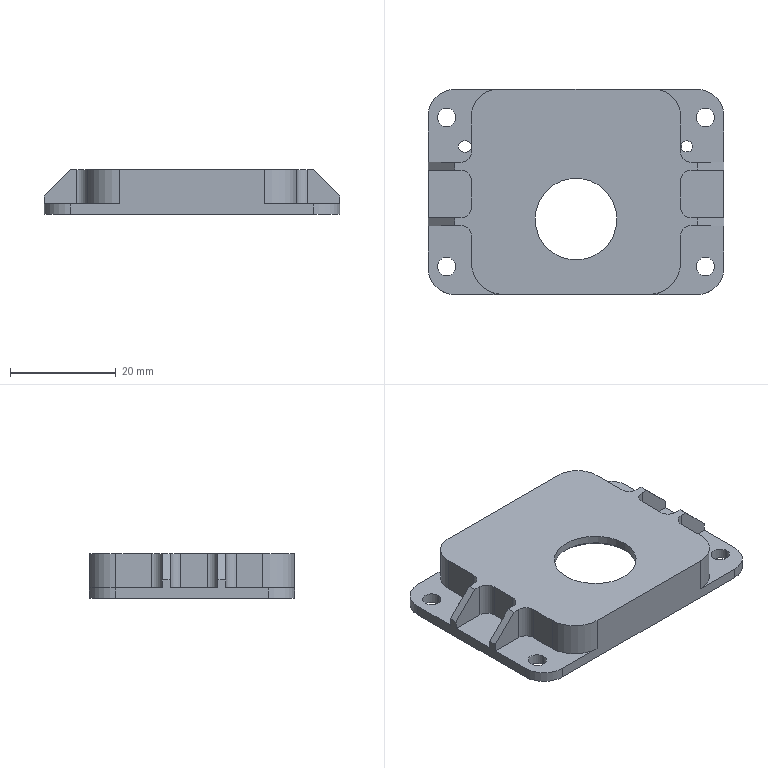NC program | NX | posted with a generic post | part box 56 x 38.85 x 8.5 mm
Lines 2523 to 3190 of 3190:
(ZLEVEL_PROFILE_COPY , TOOL : D1.5)
N5008 T20 M6
N5010 G54
N5012 G17 G0 G90 X21.294 Y8.344 S9500 M3
N5014 G43 Z30. H20
N5016 Z0.5
N5018 G94 G1 X21.435 Y8.379 Z0.492 F1000.
N5020 X21.546 Y8.537 Z0.482
N5022 Y8.646 Z0.477
N5024 X21.514 Y8.79 Z0.469
N5026 X21.432 Y8.874 Z0.463
N5028 X21.29 Y8.909 Z0.455
N5030 X21.229 Y8.925 Z0.452
N5032 X20.776 Z0.428
N5034 X20.748 Y8.916 Z0.426
N5036 X20.613 Y8.917 Z0.419
N5038 X20.521 Y8.854 Z0.413
N5040 X20.426 Y8.6 Z0.399
N5042 X20.494 Y8.427 Z0.39
N5044 X20.615 Y8.365 Z0.382
N5046 X20.775 Y8.325 Z0.374
N5048 X21.218 Z0.351
N5050 X21.435 Y8.379 Z0.339
N5052 X21.546 Y8.537 Z0.329
N5054 Y8.646 Z0.323
N5056 X21.514 Y8.79 Z0.315
N5058 X21.432 Y8.874 Z0.309
N5060 X21.29 Y8.909 Z0.301
N5062 X21.229 Y8.925 Z0.298
N5064 X20.776 Z0.274
N5066 X20.748 Y8.916 Z0.273
N5068 X20.613 Y8.917 Z0.266
N5070 X20.521 Y8.854 Z0.26
N5072 X20.426 Y8.6 Z0.246
N5074 X20.494 Y8.427 Z0.236
N5076 X20.615 Y8.365 Z0.229
N5078 X20.775 Y8.325 Z0.22
N5080 X21.218 Z0.197
N5082 X21.435 Y8.379 Z0.185
N5084 X21.546 Y8.537 Z0.175
N5086 Y8.646 Z0.169
N5088 X21.514 Y8.79 Z0.162
N5090 X21.432 Y8.874 Z0.156
N5092 X21.29 Y8.909 Z0.148
N5094 X21.229 Y8.925 Z0.145
N5096 X20.776 Z0.121
N5098 X20.748 Y8.916 Z0.119
N5100 X20.613 Y8.917 Z0.112
N5102 X20.521 Y8.854 Z0.106
N5104 X20.426 Y8.6 Z0.092
N5106 X20.494 Y8.427 Z0.082
N5108 X20.615 Y8.365 Z0.075
N5110 X20.775 Y8.325 Z0.067
N5112 X21.218 Z0.043
N5114 X21.435 Y8.379 Z0.032
N5116 X21.546 Y8.537 Z0.022
N5118 Y8.646 Z0.016
N5120 X21.514 Y8.79 Z0.008
N5122 X21.432 Y8.874 Z0.002
N5124 X21.29 Y8.909 Z-0.006
N5126 X21.229 Y8.925 Z-0.009
N5128 X20.776 Z-0.033
N5130 X20.748 Y8.916 Z-0.034
N5132 X20.613 Y8.917 Z-0.041
N5134 X20.521 Y8.854 Z-0.047
N5136 X20.426 Y8.6 Z-0.061
N5138 X20.494 Y8.427 Z-0.071
N5140 X20.615 Y8.365 Z-0.078
N5142 X20.775 Y8.325 Z-0.087
N5144 X21.026 Z-0.1
N5146 X21.218
N5148 X21.435 Y8.379
N5150 X21.546 Y8.537
N5152 Y8.646
N5154 G3 X21.29 Y8.909 R0.345
N5156 G1 X21.229 Y8.925
N5158 X20.776
N5160 X20.748 Y8.916
N5162 G3 X20.615 Y8.365 R0.291
N5164 G1 X20.775 Y8.325
N5166 X21.026
N5168 X21.258 Y8.337 Z-0.111
N5170 X21.29 Y8.343 Z-0.113
N5172 X21.456 Y8.416 Z-0.121
N5174 X21.503 Y8.475 Z-0.125
N5176 X21.543 Y8.58 Z-0.13
N5178 X21.546 Y8.63 Z-0.133
N5180 X21.527 Y8.728 Z-0.138
N5182 X21.477 Y8.807 Z-0.142
N5184 X21.449 Y8.843 Z-0.144
N5186 X21.41 Y8.865 Z-0.146
N5188 X21.327 Y8.902 Z-0.15
N5190 X21.272 Y8.911 Z-0.153
N5192 X21.062 Y8.925 Z-0.163
N5194 X20.796 Z-0.175
N5196 X20.612 Y8.879 Z-0.184
N5198 X20.548 Y8.842 Z-0.188
N5200 X20.475 Y8.732 Z-0.194
N5202 X20.457 Y8.6 Z-0.2
N5204 G3 X20.615 Y8.365 R0.291
N5206 G1 X20.775 Y8.325
N5208 X21.026
N5210 X21.257 Y8.337 Z-0.211
N5212 X21.29 Y8.343 Z-0.213
N5214 X21.456 Y8.416 Z-0.221
N5216 X21.503 Y8.475 Z-0.225
N5218 X21.543 Y8.579 Z-0.23
N5220 X21.545 Y8.663 Z-0.234
N5222 X21.527 Y8.728 Z-0.238
N5224 X21.477 Y8.81 Z-0.242
N5226 X21.447 Y8.845 Z-0.244
N5228 X21.409 Y8.866 Z-0.246
N5230 X21.327 Y8.902 Z-0.25
N5232 X21.271 Y8.911 Z-0.253
N5234 X21.062 Y8.925 Z-0.263
N5236 X20.796 Z-0.275
N5238 X20.612 Y8.879 Z-0.284
N5240 X20.549 Y8.842 Z-0.288
N5242 X20.475 Y8.731 Z-0.294
N5244 X20.457 Y8.6 Z-0.3
N5246 G3 X20.615 Y8.365 R0.291
N5248 G1 X20.775 Y8.325
N5250 X21.026
N5252 X21.257 Y8.337 Z-0.311
N5254 X21.29 Y8.343 Z-0.313
N5256 X21.455 Y8.416 Z-0.321
N5258 X21.502 Y8.475 Z-0.325
N5260 X21.546 Y8.63 Z-0.333
N5262 X21.527 Y8.728 Z-0.338
N5264 X21.48 Y8.804 Z-0.342
N5266 X21.453 Y8.839 Z-0.344
N5268 X21.414 Y8.864 Z-0.346
N5270 X21.327 Y8.902 Z-0.35
N5272 X21.27 Y8.911 Z-0.353
N5274 X21.062 Y8.925 Z-0.363
N5276 X20.796 Z-0.375
N5278 X20.612 Y8.879 Z-0.384
N5280 X20.549 Y8.841 Z-0.388
N5282 X20.475 Y8.731 Z-0.394
N5284 X20.457 Y8.6 Z-0.4
N5286 G3 X20.615 Y8.365 R0.291
N5288 G1 X20.775 Y8.325
N5290 X21.026
N5292 X21.257 Y8.337 Z-0.411
N5294 X21.29 Y8.343 Z-0.413
N5296 X21.455 Y8.416 Z-0.421
N5298 X21.502 Y8.476 Z-0.425
N5300 X21.546 Y8.629 Z-0.432
N5302 X21.527 Y8.728 Z-0.438
N5304 X21.48 Y8.804 Z-0.442
N5306 X21.453 Y8.839 Z-0.444
N5308 X21.414 Y8.863 Z-0.446
N5310 X21.327 Y8.902 Z-0.45
N5312 X21.271 Y8.912 Z-0.453
N5314 X21.062 Y8.925 Z-0.463
N5316 X20.796 Z-0.475
N5318 X20.615 Y8.879 Z-0.484
N5320 X20.55 Y8.84 Z-0.488
N5322 X20.474 Y8.73 Z-0.494
N5324 X20.451 Y8.6 Z-0.5
N5326 G3 X20.709 Y8.328 R0.3
N5328 G1 X20.775 Y8.325
N5330 X21.026
N5332 X21.259 Y8.337 Z-0.511
N5334 X21.292 Y8.343 Z-0.513
N5336 X21.411 Y8.388 Z-0.518
N5338 X21.464 Y8.415 Z-0.521
N5340 X21.51 Y8.475 Z-0.525
N5342 X21.55 Y8.635 Z-0.533
N5344 X21.529 Y8.735 Z-0.538
N5346 X21.485 Y8.811 Z-0.541
N5348 X21.457 Y8.843 Z-0.543
N5350 X21.411 Y8.863 Z-0.546
N5352 X21.32 Y8.903 Z-0.55
N5354 X21.258 Y8.914 Z-0.553
N5356 X21.054 Y8.925 Z-0.563
N5358 X20.836 Z-0.573
N5360 X20.785 Y8.92 Z-0.575
N5362 X20.59 Y8.864 Z-0.585
N5364 X20.539 Y8.839 Z-0.588
N5366 X20.468 Y8.726 Z-0.594
N5368 X20.452 Y8.594 Z-0.6
N5370 G3 X20.709 Y8.328 R0.3
N5372 G1 X20.775 Y8.325
N5374 X21.026
N5376 X21.294 Y8.343 Z-0.613
N5378 X21.456 Y8.418 Z-0.621
N5380 X21.511 Y8.477 Z-0.625
N5382 X21.547 Y8.625 Z-0.632
N5384 X21.528 Y8.738 Z-0.638
N5386 X21.456 Y8.835 Z-0.643
N5388 X21.33 Y8.901 Z-0.65
N5390 X21.281 Y8.908 Z-0.652
N5392 X21.064 Y8.925 Z-0.663
N5394 X20.794 Z-0.675
N5396 X20.61 Y8.875 Z-0.684
N5398 X20.544 Y8.843 Z-0.688
N5400 X20.47 Y8.732 Z-0.694
N5402 X20.451 Y8.599 Z-0.7
N5404 G3 X20.709 Y8.328 R0.3
N5406 G1 X20.775 Y8.325
N5408 X21.026
N5410 X21.294 Y8.343 Z-0.713
N5412 X21.456 Y8.418 Z-0.721
N5414 X21.511 Y8.477 Z-0.725
N5416 X21.547 Y8.625 Z-0.732
N5418 X21.528 Y8.738 Z-0.738
N5420 X21.456 Y8.835 Z-0.743
N5422 X21.33 Y8.901 Z-0.75
N5424 X21.281 Y8.908 Z-0.752
N5426 X21.064 Y8.925 Z-0.763
N5428 X20.794 Z-0.775
N5430 X20.61 Y8.875 Z-0.784
N5432 X20.544 Y8.843 Z-0.788
N5434 X20.47 Y8.732 Z-0.794
N5436 X20.451 Y8.599 Z-0.8
N5438 G3 X20.709 Y8.328 R0.3
N5440 G1 X20.776 Y8.325
N5442 X21.026
N5444 X21.26 Y8.338 Z-0.811
N5446 X21.294 Y8.343 Z-0.813
N5448 X21.411 Y8.388 Z-0.818
N5450 X21.465 Y8.415 Z-0.821
N5452 X21.511 Y8.477 Z-0.825
N5454 X21.55 Y8.636 Z-0.832
N5456 X21.528 Y8.738 Z-0.838
N5458 X21.457 Y8.842 Z-0.843
N5460 X21.415 Y8.862 Z-0.846
N5462 X21.33 Y8.901 Z-0.85
N5464 X21.275 Y8.909 Z-0.853
N5466 X21.064 Y8.925 Z-0.863
N5468 X20.794 Z-0.875
N5470 X20.61 Y8.875 Z-0.884
N5472 X20.544 Y8.843 Z-0.888
N5474 X20.47 Y8.732 Z-0.894
N5476 X20.451 Y8.599 Z-0.9
N5478 G3 X20.709 Y8.328 R0.3
N5480 G1 X20.776 Y8.325
N5482 X21.026
N5484 X21.26 Y8.338 Z-0.911
N5486 X21.294 Y8.343 Z-0.913
N5488 X21.411 Y8.388 Z-0.918
N5490 X21.465 Y8.415 Z-0.921
N5492 X21.511 Y8.477 Z-0.925
N5494 X21.55 Y8.636 Z-0.932
N5496 X21.528 Y8.738 Z-0.938
N5498 X21.457 Y8.842 Z-0.943
N5500 X21.415 Y8.862 Z-0.946
N5502 X21.33 Y8.901 Z-0.95
N5504 X21.275 Y8.909 Z-0.953
N5506 X21.064 Y8.925 Z-0.963
N5508 X20.794 Z-0.975
N5510 X20.61 Y8.875 Z-0.984
N5512 X20.544 Y8.843 Z-0.988
N5514 X20.47 Y8.732 Z-0.994
N5516 X20.451 Y8.599 Z-1.
N5518 G3 X20.709 Y8.328 R0.3
N5520 G1 X20.776 Y8.325
N5522 X21.026
N5524 X21.26 Y8.338 Z-1.011
N5526 X21.294 Y8.344 Z-1.013
N5528 X21.41 Y8.388 Z-1.018
N5530 X21.464 Y8.415 Z-1.021
N5532 X21.511 Y8.477 Z-1.025
N5534 X21.55 Y8.636 Z-1.032
N5536 X21.528 Y8.738 Z-1.038
N5538 X21.457 Y8.842 Z-1.043
N5540 X21.33 Y8.901 Z-1.05
N5542 X21.275 Y8.911 Z-1.053
N5544 X21.064 Y8.925 Z-1.063
N5546 X20.794 Z-1.075
N5548 X20.61 Y8.875 Z-1.084
N5550 X20.544 Y8.843 Z-1.088
N5552 X20.47 Y8.732 Z-1.094
N5554 X20.451 Y8.599 Z-1.1
N5556 G3 X20.709 Y8.328 R0.3
N5558 G1 X20.776 Y8.325
N5560 X21.026
N5562 X21.26 Y8.338 Z-1.111
N5564 X21.294 Y8.344 Z-1.113
N5566 X21.41 Y8.388 Z-1.118
N5568 X21.464 Y8.415 Z-1.121
N5570 X21.511 Y8.477 Z-1.125
N5572 X21.55 Y8.636 Z-1.132
N5574 X21.528 Y8.738 Z-1.138
N5576 X21.457 Y8.842 Z-1.143
N5578 X21.33 Y8.901 Z-1.15
N5580 X21.275 Y8.911 Z-1.153
N5582 X21.064 Y8.925 Z-1.163
N5584 X20.794 Z-1.175
N5586 X20.61 Y8.875 Z-1.184
N5588 X20.544 Y8.843 Z-1.188
N5590 X20.47 Y8.732 Z-1.194
N5592 X20.451 Y8.599 Z-1.2
N5594 G3 X20.709 Y8.328 R0.3
N5596 G1 X20.776 Y8.325
N5598 X21.026
N5600 X21.259 Y8.338 Z-1.211
N5602 X21.294 Y8.344 Z-1.213
N5604 X21.41 Y8.388 Z-1.218
N5606 X21.464 Y8.415 Z-1.221
N5608 X21.511 Y8.477 Z-1.225
N5610 X21.55 Y8.636 Z-1.232
N5612 X21.528 Y8.738 Z-1.238
N5614 X21.457 Y8.842 Z-1.243
N5616 X21.33 Y8.901 Z-1.25
N5618 X21.274 Y8.91 Z-1.253
N5620 X21.064 Y8.925 Z-1.263
N5622 X20.794 Z-1.275
N5624 X20.61 Y8.875 Z-1.284
N5626 X20.544 Y8.843 Z-1.288
N5628 X20.47 Y8.732 Z-1.294
N5630 X20.451 Y8.599 Z-1.3
N5632 G3 X20.709 Y8.328 R0.3
N5634 G1 X20.776 Y8.325
N5636 X21.026
N5638 X21.259 Y8.338 Z-1.311
N5640 X21.294 Y8.344 Z-1.313
N5642 X21.41 Y8.388 Z-1.318
N5644 X21.464 Y8.415 Z-1.321
N5646 X21.511 Y8.477 Z-1.325
N5648 X21.55 Y8.636 Z-1.332
N5650 X21.528 Y8.738 Z-1.338
N5652 X21.458 Y8.842 Z-1.343
N5654 X21.33 Y8.9 Z-1.35
N5656 X21.274 Y8.91 Z-1.353
N5658 X21.064 Y8.925 Z-1.363
N5660 X20.794 Z-1.375
N5662 X20.61 Y8.875 Z-1.384
N5664 X20.544 Y8.843 Z-1.388
N5666 X20.47 Y8.732 Z-1.394
N5668 X20.451 Y8.599 Z-1.4
N5670 G3 X20.709 Y8.328 R0.3
N5672 G1 X20.776 Y8.325
N5674 X21.026
N5676 X21.294 Y8.344 Z-1.413
N5678 X21.409 Y8.389 Z-1.418
N5680 X21.464 Y8.414 Z-1.421
N5682 X21.511 Y8.477 Z-1.425
N5684 X21.55 Y8.636 Z-1.432
N5686 X21.528 Y8.738 Z-1.438
N5688 X21.458 Y8.841 Z-1.443
N5690 X21.33 Y8.9 Z-1.45
N5692 X21.273 Y8.91 Z-1.453
N5694 X21.064 Y8.925 Z-1.463
N5696 X20.794 Z-1.475
N5698 X20.61 Y8.875 Z-1.484
N5700 X20.544 Y8.843 Z-1.488
N5702 X20.47 Y8.732 Z-1.494
N5704 X20.451 Y8.599 Z-1.5
N5706 G3 X20.709 Y8.328 R0.3
N5708 G1 X20.776 Y8.325
N5710 X21.026
N5712 X21.294 Y8.344 Z-1.513
N5714 X21.409 Y8.389 Z-1.518
N5716 X21.463 Y8.414 Z-1.521
N5718 X21.511 Y8.477 Z-1.525
N5720 X21.55 Y8.636 Z-1.532
N5722 X21.528 Y8.738 Z-1.538
N5724 X21.458 Y8.841 Z-1.543
N5726 X21.33 Y8.9 Z-1.55
N5728 X21.273 Y8.91 Z-1.553
N5730 X21.064 Y8.925 Z-1.563
N5732 X20.794 Z-1.575
N5734 X20.61 Y8.875 Z-1.584
N5736 X20.544 Y8.843 Z-1.588
N5738 X20.47 Y8.732 Z-1.594
N5740 X20.451 Y8.599 Z-1.6
N5742 G3 X20.709 Y8.328 R0.3
N5744 G1 X20.776 Y8.325
N5746 X21.026
N5748 X21.294 Y8.344 Z-1.613
N5750 X21.409 Y8.389 Z-1.618
N5752 X21.463 Y8.414 Z-1.621
N5754 X21.511 Y8.477 Z-1.625
N5756 X21.55 Y8.636 Z-1.632
N5758 X21.528 Y8.738 Z-1.638
N5760 X21.458 Y8.841 Z-1.643
N5762 X21.33 Y8.9 Z-1.65
N5764 X21.273 Y8.91 Z-1.653
N5766 X21.064 Y8.925 Z-1.663
N5768 X20.794 Z-1.675
N5770 X20.61 Y8.875 Z-1.684
N5772 X20.544 Y8.843 Z-1.688
N5774 X20.47 Y8.732 Z-1.694
N5776 X20.451 Y8.599 Z-1.7
N5778 G3 X20.709 Y8.328 R0.3
N5780 G1 X20.776 Y8.325
N5782 X21.026
N5784 X21.294 Y8.344 Z-1.713
N5786 X21.409 Y8.389 Z-1.718
N5788 X21.463 Y8.414 Z-1.721
N5790 X21.511 Y8.477 Z-1.725
N5792 X21.55 Y8.636 Z-1.732
N5794 X21.528 Y8.738 Z-1.738
N5796 X21.453 Y8.835 Z-1.743
N5798 X21.33 Y8.9 Z-1.75
N5800 X21.279 Y8.909 Z-1.752
N5802 X21.064 Y8.925 Z-1.763
N5804 X20.794 Z-1.775
N5806 X20.61 Y8.874 Z-1.784
N5808 X20.544 Y8.843 Z-1.788
N5810 X20.47 Y8.732 Z-1.794
N5812 X20.451 Y8.599 Z-1.8
N5814 G3 X20.709 Y8.328 R0.3
N5816 G1 X20.776 Y8.325
N5818 X21.026
N5820 X21.294 Y8.344 Z-1.813
N5822 X21.408 Y8.389 Z-1.818
N5824 X21.463 Y8.414 Z-1.821
N5826 X21.511 Y8.477 Z-1.825
N5828 X21.55 Y8.636 Z-1.832
N5830 X21.528 Y8.738 Z-1.838
N5832 X21.453 Y8.835 Z-1.843
N5834 X21.33 Y8.9 Z-1.85
N5836 X21.279 Y8.909 Z-1.852
N5838 X21.064 Y8.925 Z-1.863
N5840 X20.794 Z-1.875
N5842 X20.61 Y8.874 Z-1.884
N5844 X20.544 Y8.843 Z-1.888
N5846 X20.47 Y8.732 Z-1.894
N5848 X20.451 Y8.599 Z-1.9
N5850 G3 X20.709 Y8.328 R0.3
N5852 G1 X20.776 Y8.325
N5854 X21.026
N5856 X21.294 Y8.344 Z-1.913
N5858 X21.408 Y8.389 Z-1.918
N5860 X21.463 Y8.413 Z-1.921
N5862 X21.511 Y8.477 Z-1.925
N5864 X21.55 Y8.636 Z-1.932
N5866 X21.528 Y8.738 Z-1.938
N5868 X21.453 Y8.835 Z-1.943
N5870 X21.33 Y8.9 Z-1.95
N5872 X21.278 Y8.909 Z-1.952
N5874 X21.064 Y8.925 Z-1.963
N5876 X20.794 Z-1.975
N5878 X20.61 Y8.874 Z-1.984
N5880 X20.544 Y8.843 Z-1.988
N5882 X20.47 Y8.732 Z-1.994
N5884 X20.451 Y8.599 Z-2.
N5886 G3 X20.709 Y8.328 R0.3
N5888 G1 X20.776 Y8.325
N5890 X21.218
N5892 X21.292 Y8.328
N5894 G3 X21.291 Y8.922 R0.3
N5896 G1 X21.225 Y8.925
N5898 X20.748
N5900 G3 X20.451 Y8.599 R0.3
N5902 G1 Z-1.5
N5904 G0 Z30.
N5906 M5
(PLANAR_MILL_COPY_COPY_COPY_COPY_COPY_COPY_1_COPY_1_COPY_1 , TOOL : D6A45)
N5908 T01 M6
N5910 G54
N5912 G17 G0 G90 X25.2 Y-14.558 S9500 M3
N5914 G43 Z30. H1
N5916 Z0.5
N5918 G94 G1 Z-1. F1250.
N5920 G3 X25.45 Y-14.125 R0.5
N5922 X24.5 Y-13.175 R0.95
N5924 X25.45 Y-14.125 R-0.95
N5926 X25.2 Y-13.692 R0.5
N5928 G1 Z0.5
N5930 G0 Z30.
N5932 Y13.692
N5934 Z0.5
N5936 G1 Z-1.
N5938 G3 X25.45 Y14.125 R0.5
N5940 X24.5 Y15.075 R0.95
N5942 X25.45 Y14.125 R-0.95
N5944 X25.2 Y14.558 R0.5
N5946 G1 Z0.5
N5948 G0 Z30.
N5950 X-0.866 Y20.725
N5952 Z0.5
N5954 G1 Z-1.
N5956 G3 X0. Y20.225 R1.
N5958 G1 X23.
N5960 G2 X28.8 Y14.425 R5.8
N5962 G1 Y-14.425
N5964 G2 X23. Y-20.225 R5.8
N5966 G1 X-23.
N5968 G2 X-28.8 Y-14.425 R5.8
N5970 G1 Y14.425
N5972 G2 X-23. Y20.225 R5.8
N5974 G1 X0.
N5976 G3 X0.866 Y20.725 R1.
N5978 G1 Z0.5
N5980 G0 Z30.
N5982 X-25.2 Y14.558
N5984 Z0.5
N5986 G1 Z-1.
N5988 G3 X-25.45 Y14.125 R0.5
N5990 X-24.5 Y13.175 R0.95
N5992 X-25.45 Y14.125 R-0.95
N5994 X-25.2 Y13.692 R0.5
N5996 G1 Z0.5
N5998 G0 Z30.
N6000 Y-13.692
N6002 Z0.5
N6004 G1 Z-1.
N6006 G3 X-25.45 Y-14.125 R0.5
N6008 X-24.5 Y-15.075 R0.95
N6010 X-25.45 Y-14.125 R-0.95
N6012 X-25.2 Y-14.558 R0.5
N6014 G1 Z0.5
N6016 G0 Z30.
(PLANAR_MILL_COPY_COPY_COPY_COPY_COPY_COPY_1_COPY_1_COPY_1_COPY , TOOL : D6A45)
N6018 X13. Y-7.968
N6020 Z-3.
N6022 G1 Z-4.5
N6024 X13.7 Y-7.564
N6026 G3 X14.2 Y-6.698 R1.
N6028 G1 X11.4
N6030 G2 X10.4 Y-5.698 R1.
N6032 G1 Y-4.598
N6034 G2 X11.4 Y-3.598 R1.
N6036 G1 X14.2
N6038 G3 X13.7 Y-2.732 R1.
N6040 G1 Y0.186
N6042 G3 X14.2 Y1.052 R1.
N6044 G1 X11.4
N6046 G2 X10.4 Y2.052 R1.
N6048 G1 Y3.152
N6050 G2 X11.4 Y4.152 R1.
N6052 G1 X14.2
N6054 G3 X13.7 Y5.018 R1.
N6056 G1 X13. Y5.422
N6058 Z-3.
N6060 G0 Z30.
N6062 X11.57 Y12.625
N6064 Z-3.
N6066 G1 Z-4.5
N6068 X11.166 Y13.325
N6070 G3 X10.3 Y13.825 R1.
N6072 G1 Y8.025
N6074 G2 X9.3 Y7.025 R1.
N6076 G1 X8.2
N6078 G2 X7.2 Y8.025 R1.
N6080 G1 Y13.825
N6082 G3 X6.334 Y13.325 R1.
N6084 G1 X2.416
N6086 G3 X1.55 Y13.825 R1.
N6088 G1 Y8.025
N6090 G2 X0.55 Y7.025 R1.
N6092 G1 X-0.55
N6094 G2 X-1.55 Y8.025 R1.
N6096 G1 Y13.825
N6098 G3 X-2.416 Y13.325 R1.
N6100 G1 X-6.334
N6102 G3 X-7.2 Y13.825 R1.
N6104 G1 Y8.025
N6106 G2 X-8.2 Y7.025 R1.
N6108 G1 X-9.3
N6110 G2 X-10.3 Y8.025 R1.
N6112 G1 Y13.825
N6114 G3 X-11.166 Y13.325 R1.
N6116 G1 X-11.57 Y12.625
N6118 Z-3.
N6120 G0 Z30.
N6122 X-13. Y5.422
N6124 Z-3.
N6126 G1 Z-4.5
N6128 X-13.7 Y5.018
N6130 G3 X-14.2 Y4.152 R1.
N6132 G1 X-11.4
N6134 G2 X-10.4 Y3.152 R1.
N6136 G1 Y2.052
N6138 G2 X-11.4 Y1.052 R1.
N6140 G1 X-14.2
N6142 G3 X-13.7 Y0.186 R1.
N6144 G1 Y-2.732
N6146 G3 X-14.2 Y-3.598 R1.
N6148 G1 X-11.4
N6150 G2 X-10.4 Y-4.598 R1.
N6152 G1 Y-5.698
N6154 G2 X-11.4 Y-6.698 R1.
N6156 G1 X-14.2
N6158 G3 X-13.7 Y-7.564 R1.
N6160 G1 X-13. Y-7.968
N6162 Z-3.
N6164 G0 Z30.
N6166 X-11.55 Y-12.625
N6168 Z-3.
N6170 G1 Z-4.5
N6172 X-11.146 Y-13.325
N6174 G3 X-10.28 Y-13.825 R1.
N6176 G2 X-9.3 Y-13.025 R1.
N6178 G1 X-8.2
N6180 G2 X-7.22 Y-13.825 R1.
N6182 G3 X-6.354 Y-13.325 R1.
N6184 G1 X-5.95 Y-12.625
N6186 Z-3.
N6188 G0 Z30.
N6190 X5.95
N6192 Z-3.
N6194 G1 Z-4.5
N6196 X6.354 Y-13.325
N6198 G3 X7.22 Y-13.825 R1.
N6200 G2 X8.2 Y-13.025 R1.
N6202 G1 X9.3
N6204 G2 X10.28 Y-13.825 R1.
N6206 G3 X11.146 Y-13.325 R1.
N6208 G1 X11.55 Y-12.625
N6210 Z-3.
N6212 G0 Z30.
(PLANAR_MILL_COPY_COPY_COPY_COPY_COPY_COPY_1_COPY_1_COPY_1_COPY_1 , TOOL : D6A4)
N6214 X-21.3 Y9.058
N6216 Z0.5
N6218 G1 Z-1.
N6220 G3 X-21.55 Y8.625 R0.5
N6222 X-21. Y8.075 R0.55
N6224 X-21.55 Y8.625 R-0.55
N6226 X-21.3 Y8.192 R0.5
N6228 G1 Z0.5
N6230 G0 Z30.
N6232 X-16.7 Y0.866
N6234 Z0.5
N6236 G1 Z-1.
N6238 G3 X-17.2 Y0. R1.
N6240 G1 Y-14.325
N6242 G3 X-14.7 Y-16.825 R2.5
N6244 G1 X14.7
N6246 G3 X17.2 Y-14.325 R2.5
N6248 G1 Y14.325
N6250 G3 X14.7 Y16.825 R2.5
N6252 G1 X-14.7
N6254 G3 X-17.2 Y14.325 R2.5
N6256 G1 Y0.
N6258 G3 X-16.7 Y-0.866 R1.
N6260 G1 Z0.5
N6262 G0 Z30.
N6264 X20.567 Y8.325
N6266 Z0.5
N6268 G1 Z-1.
N6270 G3 X21. Y8.075 R0.5
N6272 G1 X21.25
N6274 G3 X21.8 Y8.625 R0.55
N6276 X21.25 Y9.175 R0.55
N6278 G1 X20.75
N6280 G3 X20.2 Y8.625 R0.55
N6282 X20.75 Y8.075 R0.55
N6284 G1 X21.
N6286 G3 X21.433 Y8.325 R0.5
N6288 G1 Z0.5
N6290 G0 Z30.
(PLANAR_MILL_COPY_COPY_COPY_COPY_COPY_COPY_1_COPY_1_COPY_1_COPY_1_COPY , TOOL :)
N6292 X6.75 Y-6.014
N6294 Z-6.
N6296 G1 Z-7.5
N6298 G3 X7.25 Y-5.148 R1.
N6300 X0. Y2.102 R7.25
N6302 X7.25 Y-5.148 R-7.25
N6304 X6.75 Y-4.282 R1.
N6306 G1 Z-6.
N6308 G0 Z30.
N6310 M5
N6312 M2